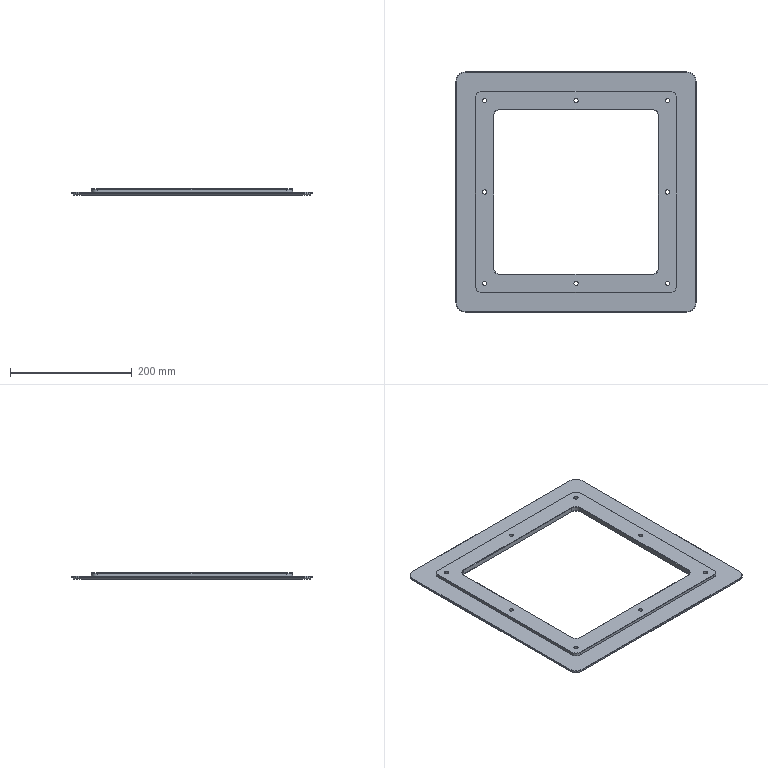NC program | Mastercam | posted with a generic post
Lines 1 to 950 of 5147:
%
O0000()
(MATERIAL - ALUMINUM MM - 2024)
( T14 | 20 FEM | H14 )
( T8 | 8 FEM | H8 | XY STOCK TO LEAVE - 0. | Z STOCK TO LEAVE - .1 )
( T12 | 12 FEM | H12 )
( T7 | 10 CHM | H7 )
( T24 | 63 FEM | H24 | XY STOCK TO LEAVE - -10. | Z STOCK TO LEAVE - 0. )
N100 G21
N110 G0 G17 G40 G49 G80 G90
N120 T14 M6
N130 G0 G90 G54 X-91.5 Y83. A0. S1600 M3
N140 G43 H14 Z50. M8
N150 Z2.
N160 G1 Z1. F600.
N170 X-89.5 F3000.
N180 G3 X-87.5 Y85. I0. J2.
N190 X-95. Y92.5 Z.925 I-7.5 J0.
N200 X-102.5 Y85. Z.85 I0. J-7.5
N210 X-95. Y77.5 Z.775 I7.5 J0.
N220 X-87.5 Y85. Z.7 I0. J7.5
N230 X-95. Y92.5 Z.625 I-7.5 J0.
N240 X-102.5 Y85. Z.55 I0. J-7.5
N250 X-95. Y77.5 Z.475 I7.5 J0.
N260 X-87.5 Y85. Z.4 I0. J7.5
N270 X-95. Y92.5 Z.325 I-7.5 J0.
N280 X-102.5 Y85. Z.25 I0. J-7.5
N290 X-95. Y77.5 Z.175 I7.5 J0.
N300 X-87.5 Y85. Z.1 I0. J7.5
N310 X-95. Y92.5 Z.025 I-7.5 J0.
N320 X-102.5 Y85. Z-.05 I0. J-7.5
N330 X-95. Y77.5 Z-.125 I7.5 J0.
N340 X-87.5 Y85. Z-.2 I0. J7.5
N350 X-95. Y92.5 Z-.275 I-7.5 J0.
N360 X-102.5 Y85. Z-.35 I0. J-7.5
N370 X-95. Y77.5 Z-.425 I7.5 J0.
N380 X-87.5 Y85. Z-.5 I0. J7.5
N390 X-95. Y92.5 Z-.575 I-7.5 J0.
N400 X-102.5 Y85. Z-.65 I0. J-7.5
N410 X-95. Y77.5 Z-.725 I7.5 J0.
N420 X-87.5 Y85. Z-.8 I0. J7.5
N430 X-95. Y92.5 Z-.875 I-7.5 J0.
N440 X-102.5 Y85. Z-.95 I0. J-7.5
N450 X-95. Y77.5 Z-1.025 I7.5 J0.
N460 X-87.5 Y85. Z-1.1 I0. J7.5
N470 X-95. Y92.5 Z-1.175 I-7.5 J0.
N480 X-102.5 Y85. Z-1.25 I0. J-7.5
N490 X-95. Y77.5 Z-1.325 I7.5 J0.
N500 X-87.5 Y85. Z-1.4 I0. J7.5
N510 X-95. Y92.5 Z-1.475 I-7.5 J0.
N520 X-102.5 Y85. Z-1.55 I0. J-7.5
N530 X-95. Y77.5 Z-1.625 I7.5 J0.
N540 X-87.5 Y85. Z-1.7 I0. J7.5
N550 X-95. Y92.5 Z-1.775 I-7.5 J0.
N560 X-102.5 Y85. Z-1.85 I0. J-7.5
N570 X-95. Y77.5 Z-1.925 I7.5 J0.
N580 X-87.5 Y85. Z-2. I0. J7.5
N590 X-95. Y92.5 I-7.5 J0.
N600 X-102.5 Y85. I0. J-7.5
N610 X-95. Y77.5 I7.5 J0.
N620 X-87.5 Y85. I0. J7.5
N630 X-89.5 Y87. I-2. J0.
N640 G1 X-91.5
N650 G0 Z50.
N660 Y-87.
N670 Z2.
N680 G1 Z1. F600.
N690 X-89.5 F3000.
N700 G3 X-87.5 Y-85. I0. J2.
N710 X-95. Y-77.5 Z.925 I-7.5 J0.
N720 X-102.5 Y-85. Z.85 I0. J-7.5
N730 X-95. Y-92.5 Z.775 I7.5 J0.
N740 X-87.5 Y-85. Z.7 I0. J7.5
N750 X-95. Y-77.5 Z.625 I-7.5 J0.
N760 X-102.5 Y-85. Z.55 I0. J-7.5
N770 X-95. Y-92.5 Z.475 I7.5 J0.
N780 X-87.5 Y-85. Z.4 I0. J7.5
N790 X-95. Y-77.5 Z.325 I-7.5 J0.
N800 X-102.5 Y-85. Z.25 I0. J-7.5
N810 X-95. Y-92.5 Z.175 I7.5 J0.
N820 X-87.5 Y-85. Z.1 I0. J7.5
N830 X-95. Y-77.5 Z.025 I-7.5 J0.
N840 X-102.5 Y-85. Z-.05 I0. J-7.5
N850 X-95. Y-92.5 Z-.125 I7.5 J0.
N860 X-87.5 Y-85. Z-.2 I0. J7.5
N870 X-95. Y-77.5 Z-.275 I-7.5 J0.
N880 X-102.5 Y-85. Z-.35 I0. J-7.5
N890 X-95. Y-92.5 Z-.425 I7.5 J0.
N900 X-87.5 Y-85. Z-.5 I0. J7.5
N910 X-95. Y-77.5 Z-.575 I-7.5 J0.
N920 X-102.5 Y-85. Z-.65 I0. J-7.5
N930 X-95. Y-92.5 Z-.725 I7.5 J0.
N940 X-87.5 Y-85. Z-.8 I0. J7.5
N950 X-95. Y-77.5 Z-.875 I-7.5 J0.
N960 X-102.5 Y-85. Z-.95 I0. J-7.5
N970 X-95. Y-92.5 Z-1.025 I7.5 J0.
N980 X-87.5 Y-85. Z-1.1 I0. J7.5
N990 X-95. Y-77.5 Z-1.175 I-7.5 J0.
N1000 X-102.5 Y-85. Z-1.25 I0. J-7.5
N1010 X-95. Y-92.5 Z-1.325 I7.5 J0.
N1020 X-87.5 Y-85. Z-1.4 I0. J7.5
N1030 X-95. Y-77.5 Z-1.475 I-7.5 J0.
N1040 X-102.5 Y-85. Z-1.55 I0. J-7.5
N1050 X-95. Y-92.5 Z-1.625 I7.5 J0.
N1060 X-87.5 Y-85. Z-1.7 I0. J7.5
N1070 X-95. Y-77.5 Z-1.775 I-7.5 J0.
N1080 X-102.5 Y-85. Z-1.85 I0. J-7.5
N1090 X-95. Y-92.5 Z-1.925 I7.5 J0.
N1100 X-87.5 Y-85. Z-2. I0. J7.5
N1110 X-95. Y-77.5 I-7.5 J0.
N1120 X-102.5 Y-85. I0. J-7.5
N1130 X-95. Y-92.5 I7.5 J0.
N1140 X-87.5 Y-85. I0. J7.5
N1150 X-89.5 Y-83. I-2. J0.
N1160 G1 X-91.5
N1170 G0 Z50.
N1180 X98.5 Y-87.
N1190 Z2.
N1200 G1 Z1. F600.
N1210 X100.5 F3000.
N1220 G3 X102.5 Y-85. I0. J2.
N1230 X95. Y-77.5 Z.925 I-7.5 J0.
N1240 X87.5 Y-85. Z.85 I0. J-7.5
N1250 X95. Y-92.5 Z.775 I7.5 J0.
N1260 X102.5 Y-85. Z.7 I0. J7.5
N1270 X95. Y-77.5 Z.625 I-7.5 J0.
N1280 X87.5 Y-85. Z.55 I0. J-7.5
N1290 X95. Y-92.5 Z.475 I7.5 J0.
N1300 X102.5 Y-85. Z.4 I0. J7.5
N1310 X95. Y-77.5 Z.325 I-7.5 J0.
N1320 X87.5 Y-85. Z.25 I0. J-7.5
N1330 X95. Y-92.5 Z.175 I7.5 J0.
N1340 X102.5 Y-85. Z.1 I0. J7.5
N1350 X95. Y-77.5 Z.025 I-7.5 J0.
N1360 X87.5 Y-85. Z-.05 I0. J-7.5
N1370 X95. Y-92.5 Z-.125 I7.5 J0.
N1380 X102.5 Y-85. Z-.2 I0. J7.5
N1390 X95. Y-77.5 Z-.275 I-7.5 J0.
N1400 X87.5 Y-85. Z-.35 I0. J-7.5
N1410 X95. Y-92.5 Z-.425 I7.5 J0.
N1420 X102.5 Y-85. Z-.5 I0. J7.5
N1430 X95. Y-77.5 Z-.575 I-7.5 J0.
N1440 X87.5 Y-85. Z-.65 I0. J-7.5
N1450 X95. Y-92.5 Z-.725 I7.5 J0.
N1460 X102.5 Y-85. Z-.8 I0. J7.5
N1470 X95. Y-77.5 Z-.875 I-7.5 J0.
N1480 X87.5 Y-85. Z-.95 I0. J-7.5
N1490 X95. Y-92.5 Z-1.025 I7.5 J0.
N1500 X102.5 Y-85. Z-1.1 I0. J7.5
N1510 X95. Y-77.5 Z-1.175 I-7.5 J0.
N1520 X87.5 Y-85. Z-1.25 I0. J-7.5
N1530 X95. Y-92.5 Z-1.325 I7.5 J0.
N1540 X102.5 Y-85. Z-1.4 I0. J7.5
N1550 X95. Y-77.5 Z-1.475 I-7.5 J0.
N1560 X87.5 Y-85. Z-1.55 I0. J-7.5
N1570 X95. Y-92.5 Z-1.625 I7.5 J0.
N1580 X102.5 Y-85. Z-1.7 I0. J7.5
N1590 X95. Y-77.5 Z-1.775 I-7.5 J0.
N1600 X87.5 Y-85. Z-1.85 I0. J-7.5
N1610 X95. Y-92.5 Z-1.925 I7.5 J0.
N1620 X102.5 Y-85. Z-2. I0. J7.5
N1630 X95. Y-77.5 I-7.5 J0.
N1640 X87.5 Y-85. I0. J-7.5
N1650 X95. Y-92.5 I7.5 J0.
N1660 X102.5 Y-85. I0. J7.5
N1670 X100.5 Y-83. I-2. J0.
N1680 G1 X98.5
N1690 G0 Z50.
N1700 Y83.
N1710 Z2.
N1720 G1 Z1. F600.
N1730 X100.5 F3000.
N1740 G3 X102.5 Y85. I0. J2.
N1750 X95. Y92.5 Z.925 I-7.5 J0.
N1760 X87.5 Y85. Z.85 I0. J-7.5
N1770 X95. Y77.5 Z.775 I7.5 J0.
N1780 X102.5 Y85. Z.7 I0. J7.5
N1790 X95. Y92.5 Z.625 I-7.5 J0.
N1800 X87.5 Y85. Z.55 I0. J-7.5
N1810 X95. Y77.5 Z.475 I7.5 J0.
N1820 X102.5 Y85. Z.4 I0. J7.5
N1830 X95. Y92.5 Z.325 I-7.5 J0.
N1840 X87.5 Y85. Z.25 I0. J-7.5
N1850 X95. Y77.5 Z.175 I7.5 J0.
N1860 X102.5 Y85. Z.1 I0. J7.5
N1870 X95. Y92.5 Z.025 I-7.5 J0.
N1880 X87.5 Y85. Z-.05 I0. J-7.5
N1890 X95. Y77.5 Z-.125 I7.5 J0.
N1900 X102.5 Y85. Z-.2 I0. J7.5
N1910 X95. Y92.5 Z-.275 I-7.5 J0.
N1920 X87.5 Y85. Z-.35 I0. J-7.5
N1930 X95. Y77.5 Z-.425 I7.5 J0.
N1940 X102.5 Y85. Z-.5 I0. J7.5
N1950 X95. Y92.5 Z-.575 I-7.5 J0.
N1960 X87.5 Y85. Z-.65 I0. J-7.5
N1970 X95. Y77.5 Z-.725 I7.5 J0.
N1980 X102.5 Y85. Z-.8 I0. J7.5
N1990 X95. Y92.5 Z-.875 I-7.5 J0.
N2000 X87.5 Y85. Z-.95 I0. J-7.5
N2010 X95. Y77.5 Z-1.025 I7.5 J0.
N2020 X102.5 Y85. Z-1.1 I0. J7.5
N2030 X95. Y92.5 Z-1.175 I-7.5 J0.
N2040 X87.5 Y85. Z-1.25 I0. J-7.5
N2050 X95. Y77.5 Z-1.325 I7.5 J0.
N2060 X102.5 Y85. Z-1.4 I0. J7.5
N2070 X95. Y92.5 Z-1.475 I-7.5 J0.
N2080 X87.5 Y85. Z-1.55 I0. J-7.5
N2090 X95. Y77.5 Z-1.625 I7.5 J0.
N2100 X102.5 Y85. Z-1.7 I0. J7.5
N2110 X95. Y92.5 Z-1.775 I-7.5 J0.
N2120 X87.5 Y85. Z-1.85 I0. J-7.5
N2130 X95. Y77.5 Z-1.925 I7.5 J0.
N2140 X102.5 Y85. Z-2. I0. J7.5
N2150 X95. Y92.5 I-7.5 J0.
N2160 X87.5 Y85. I0. J-7.5
N2170 X95. Y77.5 I7.5 J0.
N2180 X102.5 Y85. I0. J7.5
N2190 X100.5 Y87. I-2. J0.
N2200 G1 X98.5
N2210 G0 Z50.
N2220 M5
N2230 G91 G28 Z0. M9
N2240 A0.
N2250 M01
N2260 T8 M6
N2270 G0 G90 G17 G54 X-94.1 Y84.2 A0. S3500 M3
N2280 G43 H8 Z50. M8
N2290 Z2.
N2300 G1 Z1. F600.
N2310 X-93.3 F1000.
N2320 G3 X-92.5 Y85. I0. J.8
N2330 X-95. Y87.5 Z.925 I-2.5 J0.
N2340 X-97.5 Y85. Z.85 I0. J-2.5
N2350 X-95. Y82.5 Z.775 I2.5 J0.
N2360 X-92.5 Y85. Z.7 I0. J2.5
N2370 X-95. Y87.5 Z.625 I-2.5 J0.
N2380 X-97.5 Y85. Z.55 I0. J-2.5
N2390 X-95. Y82.5 Z.475 I2.5 J0.
N2400 X-92.5 Y85. Z.4 I0. J2.5
N2410 X-95. Y87.5 Z.325 I-2.5 J0.
N2420 X-97.5 Y85. Z.25 I0. J-2.5
N2430 X-95. Y82.5 Z.175 I2.5 J0.
N2440 X-92.5 Y85. Z.1 I0. J2.5
N2450 X-95. Y87.5 Z.025 I-2.5 J0.
N2460 X-97.5 Y85. Z-.05 I0. J-2.5
N2470 X-95. Y82.5 Z-.125 I2.5 J0.
N2480 X-92.5 Y85. Z-.2 I0. J2.5
N2490 X-95. Y87.5 Z-.275 I-2.5 J0.
N2500 X-97.5 Y85. Z-.35 I0. J-2.5
N2510 X-95. Y82.5 Z-.425 I2.5 J0.
N2520 X-92.5 Y85. Z-.5 I0. J2.5
N2530 X-95. Y87.5 Z-.575 I-2.5 J0.
N2540 X-97.5 Y85. Z-.65 I0. J-2.5
N2550 X-95. Y82.5 Z-.725 I2.5 J0.
N2560 X-92.5 Y85. Z-.8 I0. J2.5
N2570 X-95. Y87.5 Z-.875 I-2.5 J0.
N2580 X-97.5 Y85. Z-.95 I0. J-2.5
N2590 X-95. Y82.5 Z-1.025 I2.5 J0.
N2600 X-92.5 Y85. Z-1.1 I0. J2.5
N2610 X-95. Y87.5 Z-1.175 I-2.5 J0.
N2620 X-97.5 Y85. Z-1.25 I0. J-2.5
N2630 X-95. Y82.5 Z-1.325 I2.5 J0.
N2640 X-92.5 Y85. Z-1.4 I0. J2.5
N2650 X-95. Y87.5 Z-1.475 I-2.5 J0.
N2660 X-97.5 Y85. Z-1.55 I0. J-2.5
N2670 X-95. Y82.5 Z-1.625 I2.5 J0.
N2680 X-92.5 Y85. Z-1.7 I0. J2.5
N2690 X-95. Y87.5 Z-1.775 I-2.5 J0.
N2700 X-97.5 Y85. Z-1.85 I0. J-2.5
N2710 X-95. Y82.5 Z-1.925 I2.5 J0.
N2720 X-92.5 Y85. Z-2. I0. J2.5
N2730 X-95. Y87.5 Z-2.075 I-2.5 J0.
N2740 X-97.5 Y85. Z-2.15 I0. J-2.5
N2750 X-95. Y82.5 Z-2.225 I2.5 J0.
N2760 X-92.5 Y85. Z-2.3 I0. J2.5
N2770 X-95. Y87.5 Z-2.375 I-2.5 J0.
N2780 X-97.5 Y85. Z-2.45 I0. J-2.5
N2790 X-95. Y82.5 Z-2.525 I2.5 J0.
N2800 X-92.5 Y85. Z-2.6 I0. J2.5
N2810 X-95. Y87.5 Z-2.675 I-2.5 J0.
N2820 X-97.5 Y85. Z-2.75 I0. J-2.5
N2830 X-95. Y82.5 Z-2.825 I2.5 J0.
N2840 X-92.5 Y85. Z-2.9 I0. J2.5
N2850 X-95. Y87.5 Z-2.975 I-2.5 J0.
N2860 X-97.5 Y85. Z-3.05 I0. J-2.5
N2870 X-95. Y82.5 Z-3.125 I2.5 J0.
N2880 X-92.5 Y85. Z-3.2 I0. J2.5
N2890 X-95. Y87.5 Z-3.275 I-2.5 J0.
N2900 X-97.5 Y85. Z-3.35 I0. J-2.5
N2910 X-95. Y82.5 Z-3.425 I2.5 J0.
N2920 X-92.5 Y85. Z-3.5 I0. J2.5
N2930 X-95. Y87.5 Z-3.575 I-2.5 J0.
N2940 X-97.5 Y85. Z-3.65 I0. J-2.5
N2950 X-95. Y82.5 Z-3.725 I2.5 J0.
N2960 X-92.5 Y85. Z-3.8 I0. J2.5
N2970 X-95. Y87.5 Z-3.875 I-2.5 J0.
N2980 X-97.5 Y85. Z-3.95 I0. J-2.5
N2990 X-95. Y82.5 Z-4.025 I2.5 J0.
N3000 X-92.5 Y85. Z-4.1 I0. J2.5
N3010 X-95. Y87.5 Z-4.175 I-2.5 J0.
N3020 X-97.5 Y85. Z-4.25 I0. J-2.5
N3030 X-95. Y82.5 Z-4.325 I2.5 J0.
N3040 X-92.5 Y85. Z-4.4 I0. J2.5
N3050 X-95. Y87.5 Z-4.475 I-2.5 J0.
N3060 X-97.5 Y85. Z-4.55 I0. J-2.5
N3070 X-95. Y82.5 Z-4.625 I2.5 J0.
N3080 X-92.5 Y85. Z-4.7 I0. J2.5
N3090 X-95. Y87.5 Z-4.775 I-2.5 J0.
N3100 X-97.5 Y85. Z-4.85 I0. J-2.5
N3110 X-95. Y82.5 Z-4.925 I2.5 J0.
N3120 X-92.5 Y85. Z-5. I0. J2.5
N3130 X-95. Y87.5 Z-5.075 I-2.5 J0.
N3140 X-97.5 Y85. Z-5.15 I0. J-2.5
N3150 X-95. Y82.5 Z-5.225 I2.5 J0.
N3160 X-92.5 Y85. Z-5.3 I0. J2.5
N3170 X-95. Y87.5 Z-5.375 I-2.5 J0.
N3180 X-97.5 Y85. Z-5.45 I0. J-2.5
N3190 X-95. Y82.5 Z-5.525 I2.5 J0.
N3200 X-92.5 Y85. Z-5.6 I0. J2.5
N3210 X-95. Y87.5 Z-5.675 I-2.5 J0.
N3220 X-97.5 Y85. Z-5.75 I0. J-2.5
N3230 X-95. Y82.5 Z-5.825 I2.5 J0.
N3240 X-92.5 Y85. Z-5.9 I0. J2.5
N3250 X-95. Y87.5 Z-5.975 I-2.5 J0.
N3260 X-97.5 Y85. Z-6.05 I0. J-2.5
N3270 X-95. Y82.5 Z-6.125 I2.5 J0.
N3280 X-92.5 Y85. Z-6.2 I0. J2.5
N3290 X-95. Y87.5 Z-6.275 I-2.5 J0.
N3300 X-97.5 Y85. Z-6.35 I0. J-2.5
N3310 X-95. Y82.5 Z-6.425 I2.5 J0.
N3320 X-92.5 Y85. Z-6.5 I0. J2.5
N3330 X-95. Y87.5 Z-6.575 I-2.5 J0.
N3340 X-97.5 Y85. Z-6.65 I0. J-2.5
N3350 X-95. Y82.5 Z-6.725 I2.5 J0.
N3360 X-92.5 Y85. Z-6.8 I0. J2.5
N3370 X-95. Y87.5 Z-6.875 I-2.5 J0.
N3380 X-97.5 Y85. Z-6.95 I0. J-2.5
N3390 X-95. Y82.5 Z-7.025 I2.5 J0.
N3400 X-92.5 Y85. Z-7.1 I0. J2.5
N3410 X-95. Y87.5 Z-7.175 I-2.5 J0.
N3420 X-97.5 Y85. Z-7.25 I0. J-2.5
N3430 X-95. Y82.5 Z-7.325 I2.5 J0.
N3440 X-92.5 Y85. Z-7.4 I0. J2.5
N3450 X-95. Y87.5 Z-7.475 I-2.5 J0.
N3460 X-97.5 Y85. Z-7.55 I0. J-2.5
N3470 X-95. Y82.5 Z-7.625 I2.5 J0.
N3480 X-92.5 Y85. Z-7.7 I0. J2.5
N3490 X-95. Y87.5 Z-7.775 I-2.5 J0.
N3500 X-97.5 Y85. Z-7.85 I0. J-2.5
N3510 X-95. Y82.5 Z-7.925 I2.5 J0.
N3520 X-92.5 Y85. Z-8. I0. J2.5
N3530 X-95. Y87.5 Z-8.075 I-2.5 J0.
N3540 X-97.5 Y85. Z-8.15 I0. J-2.5
N3550 X-95. Y82.5 Z-8.225 I2.5 J0.
N3560 X-92.5 Y85. Z-8.3 I0. J2.5
N3570 X-95. Y87.5 Z-8.375 I-2.5 J0.
N3580 X-97.5 Y85. Z-8.45 I0. J-2.5
N3590 X-95. Y82.5 Z-8.525 I2.5 J0.
N3600 X-92.5 Y85. Z-8.6 I0. J2.5
N3610 X-95. Y87.5 Z-8.675 I-2.5 J0.
N3620 X-97.5 Y85. Z-8.75 I0. J-2.5
N3630 X-95. Y82.5 Z-8.825 I2.5 J0.
N3640 X-92.5 Y85. Z-8.9 I0. J2.5
N3650 X-95. Y87.5 Z-8.975 I-2.5 J0.
N3660 X-97.5 Y85. Z-9.05 I0. J-2.5
N3670 X-95. Y82.5 Z-9.125 I2.5 J0.
N3680 X-92.5 Y85. Z-9.2 I0. J2.5
N3690 X-95. Y87.5 Z-9.275 I-2.5 J0.
N3700 X-97.5 Y85. Z-9.35 I0. J-2.5
N3710 X-95. Y82.5 Z-9.425 I2.5 J0.
N3720 X-92.5 Y85. Z-9.5 I0. J2.5
N3730 X-95. Y87.5 Z-9.575 I-2.5 J0.
N3740 X-97.5 Y85. Z-9.65 I0. J-2.5
N3750 X-95. Y82.5 Z-9.725 I2.5 J0.
N3760 X-92.5 Y85. Z-9.8 I0. J2.5
N3770 X-95. Y87.5 Z-9.875 I-2.5 J0.
N3780 X-97.5 Y85. Z-9.95 I0. J-2.5
N3790 X-95. Y82.5 Z-10.025 I2.5 J0.
N3800 X-92.5 Y85. Z-10.1 I0. J2.5
N3810 X-95. Y87.5 Z-10.175 I-2.5 J0.
N3820 X-97.5 Y85. Z-10.25 I0. J-2.5
N3830 X-95. Y82.5 Z-10.325 I2.5 J0.
N3840 X-92.5 Y85. Z-10.4 I0. J2.5
N3850 X-95. Y87.5 Z-10.475 I-2.5 J0.
N3860 X-97.5 Y85. Z-10.55 I0. J-2.5
N3870 X-95. Y82.5 Z-10.625 I2.5 J0.
N3880 X-92.5 Y85. Z-10.7 I0. J2.5
N3890 X-95. Y87.5 Z-10.775 I-2.5 J0.
N3900 X-97.5 Y85. Z-10.85 I0. J-2.5
N3910 X-95. Y82.5 Z-10.925 I2.5 J0.
N3920 X-92.5 Y85. Z-11. I0. J2.5
N3930 X-95. Y87.5 Z-11.075 I-2.5 J0.
N3940 X-97.5 Y85. Z-11.15 I0. J-2.5
N3950 X-95. Y82.5 Z-11.225 I2.5 J0.
N3960 X-92.5 Y85. Z-11.3 I0. J2.5
N3970 X-95. Y87.5 Z-11.375 I-2.5 J0.
N3980 X-96.25 Y87.165 Z-11.4 I0. J-2.5
N3990 X-97.5 Y85. I1.25 J-2.165
N4000 X-95. Y82.5 I2.5 J0.
N4010 X-92.5 Y85. I0. J2.5
N4020 X-95. Y87.5 I-2.5 J0.
N4030 X-96.25 Y87.165 I0. J-2.5
N4040 X-96.65 Y86.472 I.4 J-.693
N4050 X-96.543 Y86.072 I.8 J0.
N4060 G1 X-96.143 Y85.379
N4070 G0 Z50.
N4080 X95.9 Y-85.8
N4090 Z2.
N4100 G1 Z1. F600.
N4110 X96.7 F1000.
N4120 G3 X97.5 Y-85. I0. J.8
N4130 X95. Y-82.5 Z.925 I-2.5 J0.
N4140 X92.5 Y-85. Z.85 I0. J-2.5
N4150 X95. Y-87.5 Z.775 I2.5 J0.
N4160 X97.5 Y-85. Z.7 I0. J2.5
N4170 X95. Y-82.5 Z.625 I-2.5 J0.
N4180 X92.5 Y-85. Z.55 I0. J-2.5
N4190 X95. Y-87.5 Z.475 I2.5 J0.
N4200 X97.5 Y-85. Z.4 I0. J2.5
N4210 X95. Y-82.5 Z.325 I-2.5 J0.
N4220 X92.5 Y-85. Z.25 I0. J-2.5
N4230 X95. Y-87.5 Z.175 I2.5 J0.
N4240 X97.5 Y-85. Z.1 I0. J2.5
N4250 X95. Y-82.5 Z.025 I-2.5 J0.
N4260 X92.5 Y-85. Z-.05 I0. J-2.5
N4270 X95. Y-87.5 Z-.125 I2.5 J0.
N4280 X97.5 Y-85. Z-.2 I0. J2.5
N4290 X95. Y-82.5 Z-.275 I-2.5 J0.
N4300 X92.5 Y-85. Z-.35 I0. J-2.5
N4310 X95. Y-87.5 Z-.425 I2.5 J0.
N4320 X97.5 Y-85. Z-.5 I0. J2.5
N4330 X95. Y-82.5 Z-.575 I-2.5 J0.
N4340 X92.5 Y-85. Z-.65 I0. J-2.5
N4350 X95. Y-87.5 Z-.725 I2.5 J0.
N4360 X97.5 Y-85. Z-.8 I0. J2.5
N4370 X95. Y-82.5 Z-.875 I-2.5 J0.
N4380 X92.5 Y-85. Z-.95 I0. J-2.5
N4390 X95. Y-87.5 Z-1.025 I2.5 J0.
N4400 X97.5 Y-85. Z-1.1 I0. J2.5
N4410 X95. Y-82.5 Z-1.175 I-2.5 J0.
N4420 X92.5 Y-85. Z-1.25 I0. J-2.5
N4430 X95. Y-87.5 Z-1.325 I2.5 J0.
N4440 X97.5 Y-85. Z-1.4 I0. J2.5
N4450 X95. Y-82.5 Z-1.475 I-2.5 J0.
N4460 X92.5 Y-85. Z-1.55 I0. J-2.5
N4470 X95. Y-87.5 Z-1.625 I2.5 J0.
N4480 X97.5 Y-85. Z-1.7 I0. J2.5
N4490 X95. Y-82.5 Z-1.775 I-2.5 J0.
N4500 X92.5 Y-85. Z-1.85 I0. J-2.5
N4510 X95. Y-87.5 Z-1.925 I2.5 J0.
N4520 X97.5 Y-85. Z-2. I0. J2.5
N4530 X95. Y-82.5 Z-2.075 I-2.5 J0.
N4540 X92.5 Y-85. Z-2.15 I0. J-2.5
N4550 X95. Y-87.5 Z-2.225 I2.5 J0.
N4560 X97.5 Y-85. Z-2.3 I0. J2.5
N4570 X95. Y-82.5 Z-2.375 I-2.5 J0.
N4580 X92.5 Y-85. Z-2.45 I0. J-2.5
N4590 X95. Y-87.5 Z-2.525 I2.5 J0.
N4600 X97.5 Y-85. Z-2.6 I0. J2.5
N4610 X95. Y-82.5 Z-2.675 I-2.5 J0.
N4620 X92.5 Y-85. Z-2.75 I0. J-2.5
N4630 X95. Y-87.5 Z-2.825 I2.5 J0.
N4640 X97.5 Y-85. Z-2.9 I0. J2.5
N4650 X95. Y-82.5 Z-2.975 I-2.5 J0.
N4660 X92.5 Y-85. Z-3.05 I0. J-2.5
N4670 X95. Y-87.5 Z-3.125 I2.5 J0.
N4680 X97.5 Y-85. Z-3.2 I0. J2.5
N4690 X95. Y-82.5 Z-3.275 I-2.5 J0.
N4700 X92.5 Y-85. Z-3.35 I0. J-2.5
N4710 X95. Y-87.5 Z-3.425 I2.5 J0.
N4720 X97.5 Y-85. Z-3.5 I0. J2.5
N4730 X95. Y-82.5 Z-3.575 I-2.5 J0.
N4740 X92.5 Y-85. Z-3.65 I0. J-2.5
N4750 X95. Y-87.5 Z-3.725 I2.5 J0.
N4760 X97.5 Y-85. Z-3.8 I0. J2.5
N4770 X95. Y-82.5 Z-3.875 I-2.5 J0.
N4780 X92.5 Y-85. Z-3.95 I0. J-2.5
N4790 X95. Y-87.5 Z-4.025 I2.5 J0.
N4800 X97.5 Y-85. Z-4.1 I0. J2.5
N4810 X95. Y-82.5 Z-4.175 I-2.5 J0.
N4820 X92.5 Y-85. Z-4.25 I0. J-2.5
N4830 X95. Y-87.5 Z-4.325 I2.5 J0.
N4840 X97.5 Y-85. Z-4.4 I0. J2.5
N4850 X95. Y-82.5 Z-4.475 I-2.5 J0.
N4860 X92.5 Y-85. Z-4.55 I0. J-2.5
N4870 X95. Y-87.5 Z-4.625 I2.5 J0.
N4880 X97.5 Y-85. Z-4.7 I0. J2.5
N4890 X95. Y-82.5 Z-4.775 I-2.5 J0.
N4900 X92.5 Y-85. Z-4.85 I0. J-2.5
N4910 X95. Y-87.5 Z-4.925 I2.5 J0.
N4920 X97.5 Y-85. Z-5. I0. J2.5
N4930 X95. Y-82.5 Z-5.075 I-2.5 J0.
N4940 X92.5 Y-85. Z-5.15 I0. J-2.5
N4950 X95. Y-87.5 Z-5.225 I2.5 J0.
N4960 X97.5 Y-85. Z-5.3 I0. J2.5
N4970 X95. Y-82.5 Z-5.375 I-2.5 J0.
N4980 X92.5 Y-85. Z-5.45 I0. J-2.5
N4990 X95. Y-87.5 Z-5.525 I2.5 J0.
N5000 X97.5 Y-85. Z-5.6 I0. J2.5
N5010 X95. Y-82.5 Z-5.675 I-2.5 J0.
N5020 X92.5 Y-85. Z-5.75 I0. J-2.5
N5030 X95. Y-87.5 Z-5.825 I2.5 J0.
N5040 X97.5 Y-85. Z-5.9 I0. J2.5
N5050 X95. Y-82.5 Z-5.975 I-2.5 J0.
N5060 X92.5 Y-85. Z-6.05 I0. J-2.5
N5070 X95. Y-87.5 Z-6.125 I2.5 J0.
N5080 X97.5 Y-85. Z-6.2 I0. J2.5
N5090 X95. Y-82.5 Z-6.275 I-2.5 J0.
N5100 X92.5 Y-85. Z-6.35 I0. J-2.5
N5110 X95. Y-87.5 Z-6.425 I2.5 J0.
N5120 X97.5 Y-85. Z-6.5 I0. J2.5
N5130 X95. Y-82.5 Z-6.575 I-2.5 J0.
N5140 X92.5 Y-85. Z-6.65 I0. J-2.5
N5150 X95. Y-87.5 Z-6.725 I2.5 J0.
N5160 X97.5 Y-85. Z-6.8 I0. J2.5
N5170 X95. Y-82.5 Z-6.875 I-2.5 J0.
N5180 X92.5 Y-85. Z-6.95 I0. J-2.5
N5190 X95. Y-87.5 Z-7.025 I2.5 J0.
N5200 X97.5 Y-85. Z-7.1 I0. J2.5
N5210 X95. Y-82.5 Z-7.175 I-2.5 J0.
N5220 X92.5 Y-85. Z-7.25 I0. J-2.5
N5230 X95. Y-87.5 Z-7.325 I2.5 J0.
N5240 X97.5 Y-85. Z-7.4 I0. J2.5
N5250 X95. Y-82.5 Z-7.475 I-2.5 J0.
N5260 X92.5 Y-85. Z-7.55 I0. J-2.5
N5270 X95. Y-87.5 Z-7.625 I2.5 J0.
N5280 X97.5 Y-85. Z-7.7 I0. J2.5
N5290 X95. Y-82.5 Z-7.775 I-2.5 J0.
N5300 X92.5 Y-85. Z-7.85 I0. J-2.5
N5310 X95. Y-87.5 Z-7.925 I2.5 J0.
N5320 X97.5 Y-85. Z-8. I0. J2.5
N5330 X95. Y-82.5 Z-8.075 I-2.5 J0.
N5340 X92.5 Y-85. Z-8.15 I0. J-2.5
N5350 X95. Y-87.5 Z-8.225 I2.5 J0.
N5360 X97.5 Y-85. Z-8.3 I0. J2.5
N5370 X95. Y-82.5 Z-8.375 I-2.5 J0.
N5380 X92.5 Y-85. Z-8.45 I0. J-2.5
N5390 X95. Y-87.5 Z-8.525 I2.5 J0.
N5400 X97.5 Y-85. Z-8.6 I0. J2.5
N5410 X95. Y-82.5 Z-8.675 I-2.5 J0.
N5420 X92.5 Y-85. Z-8.75 I0. J-2.5
N5430 X95. Y-87.5 Z-8.825 I2.5 J0.
N5440 X97.5 Y-85. Z-8.9 I0. J2.5
N5450 X95. Y-82.5 Z-8.975 I-2.5 J0.
N5460 X92.5 Y-85. Z-9.05 I0. J-2.5
N5470 X95. Y-87.5 Z-9.125 I2.5 J0.
N5480 X97.5 Y-85. Z-9.2 I0. J2.5
N5490 X95. Y-82.5 Z-9.275 I-2.5 J0.
N5500 X92.5 Y-85. Z-9.35 I0. J-2.5
N5510 X95. Y-87.5 Z-9.425 I2.5 J0.
N5520 X97.5 Y-85. Z-9.5 I0. J2.5
N5530 X95. Y-82.5 Z-9.575 I-2.5 J0.
N5540 X92.5 Y-85. Z-9.65 I0. J-2.5
N5550 X95. Y-87.5 Z-9.725 I2.5 J0.
N5560 X97.5 Y-85. Z-9.8 I0. J2.5
N5570 X95. Y-82.5 Z-9.875 I-2.5 J0.
N5580 X92.5 Y-85. Z-9.95 I0. J-2.5
N5590 X95. Y-87.5 Z-10.025 I2.5 J0.
N5600 X97.5 Y-85. Z-10.1 I0. J2.5
N5610 X95. Y-82.5 Z-10.175 I-2.5 J0.
N5620 X92.5 Y-85. Z-10.25 I0. J-2.5
N5630 X95. Y-87.5 Z-10.325 I2.5 J0.
N5640 X97.5 Y-85. Z-10.4 I0. J2.5
N5650 X95. Y-82.5 Z-10.475 I-2.5 J0.
N5660 X92.5 Y-85. Z-10.55 I0. J-2.5
N5670 X95. Y-87.5 Z-10.625 I2.5 J0.
N5680 X97.5 Y-85. Z-10.7 I0. J2.5
N5690 X95. Y-82.5 Z-10.775 I-2.5 J0.
N5700 X92.5 Y-85. Z-10.85 I0. J-2.5
N5710 X95. Y-87.5 Z-10.925 I2.5 J0.
N5720 X97.5 Y-85. Z-11. I0. J2.5
N5730 X95. Y-82.5 Z-11.075 I-2.5 J0.
N5740 X92.5 Y-85. Z-11.15 I0. J-2.5
N5750 X95. Y-87.5 Z-11.225 I2.5 J0.
N5760 X97.5 Y-85. Z-11.3 I0. J2.5
N5770 X95. Y-82.5 Z-11.375 I-2.5 J0.
N5780 X93.75 Y-82.835 Z-11.4 I0. J-2.5
N5790 X92.5 Y-85. I1.25 J-2.165
N5800 X95. Y-87.5 I2.5 J0.
N5810 X97.5 Y-85. I0. J2.5
N5820 X95. Y-82.5 I-2.5 J0.
N5830 X93.75 Y-82.835 I0. J-2.5
N5840 X93.35 Y-83.528 I.4 J-.693
N5850 X93.457 Y-83.928 I.8 J0.
N5860 G1 X93.857 Y-84.621
N5870 G0 Z50.
N5880 X-94.1 Y-85.8
N5890 Z2.
N5900 G1 Z1. F600.
N5910 X-93.3 F1000.
N5920 G3 X-92.5 Y-85. I0. J.8
N5930 X-95. Y-82.5 Z.925 I-2.5 J0.
N5940 X-97.5 Y-85. Z.85 I0. J-2.5
N5950 X-95. Y-87.5 Z.775 I2.5 J0.
N5960 X-92.5 Y-85. Z.7 I0. J2.5
N5970 X-95. Y-82.5 Z.625 I-2.5 J0.
N5980 X-97.5 Y-85. Z.55 I0. J-2.5
N5990 X-95. Y-87.5 Z.475 I2.5 J0.
N6000 X-92.5 Y-85. Z.4 I0. J2.5
N6010 X-95. Y-82.5 Z.325 I-2.5 J0.
N6020 X-97.5 Y-85. Z.25 I0. J-2.5
N6030 X-95. Y-87.5 Z.175 I2.5 J0.
N6040 X-92.5 Y-85. Z.1 I0. J2.5
N6050 X-95. Y-82.5 Z.025 I-2.5 J0.
N6060 X-97.5 Y-85. Z-.05 I0. J-2.5
N6070 X-95. Y-87.5 Z-.125 I2.5 J0.
N6080 X-92.5 Y-85. Z-.2 I0. J2.5
N6090 X-95. Y-82.5 Z-.275 I-2.5 J0.
N6100 X-97.5 Y-85. Z-.35 I0. J-2.5
N6110 X-95. Y-87.5 Z-.425 I2.5 J0.
N6120 X-92.5 Y-85. Z-.5 I0. J2.5
N6130 X-95. Y-82.5 Z-.575 I-2.5 J0.
N6140 X-97.5 Y-85. Z-.65 I0. J-2.5
N6150 X-95. Y-87.5 Z-.725 I2.5 J0.
N6160 X-92.5 Y-85. Z-.8 I0. J2.5
N6170 X-95. Y-82.5 Z-.875 I-2.5 J0.
N6180 X-97.5 Y-85. Z-.95 I0. J-2.5
N6190 X-95. Y-87.5 Z-1.025 I2.5 J0.
N6200 X-92.5 Y-85. Z-1.1 I0. J2.5
N6210 X-95. Y-82.5 Z-1.175 I-2.5 J0.
N6220 X-97.5 Y-85. Z-1.25 I0. J-2.5
N6230 X-95. Y-87.5 Z-1.325 I2.5 J0.
N6240 X-92.5 Y-85. Z-1.4 I0. J2.5
N6250 X-95. Y-82.5 Z-1.475 I-2.5 J0.
N6260 X-97.5 Y-85. Z-1.55 I0. J-2.5
N6270 X-95. Y-87.5 Z-1.625 I2.5 J0.
N6280 X-92.5 Y-85. Z-1.7 I0. J2.5
N6290 X-95. Y-82.5 Z-1.775 I-2.5 J0.
N6300 X-97.5 Y-85. Z-1.85 I0. J-2.5
N6310 X-95. Y-87.5 Z-1.925 I2.5 J0.
N6320 X-92.5 Y-85. Z-2. I0. J2.5
N6330 X-95. Y-82.5 Z-2.075 I-2.5 J0.
N6340 X-97.5 Y-85. Z-2.15 I0. J-2.5
N6350 X-95. Y-87.5 Z-2.225 I2.5 J0.
N6360 X-92.5 Y-85. Z-2.3 I0. J2.5
N6370 X-95. Y-82.5 Z-2.375 I-2.5 J0.
N6380 X-97.5 Y-85. Z-2.45 I0. J-2.5
N6390 X-95. Y-87.5 Z-2.525 I2.5 J0.
N6400 X-92.5 Y-85. Z-2.6 I0. J2.5
N6410 X-95. Y-82.5 Z-2.675 I-2.5 J0.
N6420 X-97.5 Y-85. Z-2.75 I0. J-2.5
N6430 X-95. Y-87.5 Z-2.825 I2.5 J0.
N6440 X-92.5 Y-85. Z-2.9 I0. J2.5
N6450 X-95. Y-82.5 Z-2.975 I-2.5 J0.
N6460 X-97.5 Y-85. Z-3.05 I0. J-2.5
N6470 X-95. Y-87.5 Z-3.125 I2.5 J0.
N6480 X-92.5 Y-85. Z-3.2 I0. J2.5
N6490 X-95. Y-82.5 Z-3.275 I-2.5 J0.
N6500 X-97.5 Y-85. Z-3.35 I0. J-2.5
N6510 X-95. Y-87.5 Z-3.425 I2.5 J0.
N6520 X-92.5 Y-85. Z-3.5 I0. J2.5
N6530 X-95. Y-82.5 Z-3.575 I-2.5 J0.
N6540 X-97.5 Y-85. Z-3.65 I0. J-2.5
N6550 X-95. Y-87.5 Z-3.725 I2.5 J0.
N6560 X-92.5 Y-85. Z-3.8 I0. J2.5
N6570 X-95. Y-82.5 Z-3.875 I-2.5 J0.
N6580 X-97.5 Y-85. Z-3.95 I0. J-2.5
N6590 X-95. Y-87.5 Z-4.025 I2.5 J0.
N6600 X-92.5 Y-85. Z-4.1 I0. J2.5
N6610 X-95. Y-82.5 Z-4.175 I-2.5 J0.
N6620 X-97.5 Y-85. Z-4.25 I0. J-2.5
N6630 X-95. Y-87.5 Z-4.325 I2.5 J0.
N6640 X-92.5 Y-85. Z-4.4 I0. J2.5
N6650 X-95. Y-82.5 Z-4.475 I-2.5 J0.
N6660 X-97.5 Y-85. Z-4.55 I0. J-2.5
N6670 X-95. Y-87.5 Z-4.625 I2.5 J0.
N6680 X-92.5 Y-85. Z-4.7 I0. J2.5
N6690 X-95. Y-82.5 Z-4.775 I-2.5 J0.
N6700 X-97.5 Y-85. Z-4.85 I0. J-2.5
N6710 X-95. Y-87.5 Z-4.925 I2.5 J0.
N6720 X-92.5 Y-85. Z-5. I0. J2.5
N6730 X-95. Y-82.5 Z-5.075 I-2.5 J0.
N6740 X-97.5 Y-85. Z-5.15 I0. J-2.5
N6750 X-95. Y-87.5 Z-5.225 I2.5 J0.
N6760 X-92.5 Y-85. Z-5.3 I0. J2.5
N6770 X-95. Y-82.5 Z-5.375 I-2.5 J0.
N6780 X-97.5 Y-85. Z-5.45 I0. J-2.5
N6790 X-95. Y-87.5 Z-5.525 I2.5 J0.
N6800 X-92.5 Y-85. Z-5.6 I0. J2.5
N6810 X-95. Y-82.5 Z-5.675 I-2.5 J0.
N6820 X-97.5 Y-85. Z-5.75 I0. J-2.5
N6830 X-95. Y-87.5 Z-5.825 I2.5 J0.
N6840 X-92.5 Y-85. Z-5.9 I0. J2.5
N6850 X-95. Y-82.5 Z-5.975 I-2.5 J0.
N6860 X-97.5 Y-85. Z-6.05 I0. J-2.5
N6870 X-95. Y-87.5 Z-6.125 I2.5 J0.
N6880 X-92.5 Y-85. Z-6.2 I0. J2.5
N6890 X-95. Y-82.5 Z-6.275 I-2.5 J0.
N6900 X-97.5 Y-85. Z-6.35 I0. J-2.5
N6910 X-95. Y-87.5 Z-6.425 I2.5 J0.
N6920 X-92.5 Y-85. Z-6.5 I0. J2.5
N6930 X-95. Y-82.5 Z-6.575 I-2.5 J0.
N6940 X-97.5 Y-85. Z-6.65 I0. J-2.5
N6950 X-95. Y-87.5 Z-6.725 I2.5 J0.
N6960 X-92.5 Y-85. Z-6.8 I0. J2.5
N6970 X-95. Y-82.5 Z-6.875 I-2.5 J0.
N6980 X-97.5 Y-85. Z-6.95 I0. J-2.5
N6990 X-95. Y-87.5 Z-7.025 I2.5 J0.
N7000 X-92.5 Y-85. Z-7.1 I0. J2.5
N7010 X-95. Y-82.5 Z-7.175 I-2.5 J0.
N7020 X-97.5 Y-85. Z-7.25 I0. J-2.5
N7030 X-95. Y-87.5 Z-7.325 I2.5 J0.
N7040 X-92.5 Y-85. Z-7.4 I0. J2.5
N7050 X-95. Y-82.5 Z-7.475 I-2.5 J0.
N7060 X-97.5 Y-85. Z-7.55 I0. J-2.5
N7070 X-95. Y-87.5 Z-7.625 I2.5 J0.
N7080 X-92.5 Y-85. Z-7.7 I0. J2.5
N7090 X-95. Y-82.5 Z-7.775 I-2.5 J0.
N7100 X-97.5 Y-85. Z-7.85 I0. J-2.5
N7110 X-95. Y-87.5 Z-7.925 I2.5 J0.
N7120 X-92.5 Y-85. Z-8. I0. J2.5
N7130 X-95. Y-82.5 Z-8.075 I-2.5 J0.
N7140 X-97.5 Y-85. Z-8.15 I0. J-2.5
N7150 X-95. Y-87.5 Z-8.225 I2.5 J0.
N7160 X-92.5 Y-85. Z-8.3 I0. J2.5
N7170 X-95. Y-82.5 Z-8.375 I-2.5 J0.
N7180 X-97.5 Y-85. Z-8.45 I0. J-2.5
N7190 X-95. Y-87.5 Z-8.525 I2.5 J0.
N7200 X-92.5 Y-85. Z-8.6 I0. J2.5
N7210 X-95. Y-82.5 Z-8.675 I-2.5 J0.
N7220 X-97.5 Y-85. Z-8.75 I0. J-2.5
N7230 X-95. Y-87.5 Z-8.825 I2.5 J0.
N7240 X-92.5 Y-85. Z-8.9 I0. J2.5
N7250 X-95. Y-82.5 Z-8.975 I-2.5 J0.
N7260 X-97.5 Y-85. Z-9.05 I0. J-2.5
N7270 X-95. Y-87.5 Z-9.125 I2.5 J0.
N7280 X-92.5 Y-85. Z-9.2 I0. J2.5
N7290 X-95. Y-82.5 Z-9.275 I-2.5 J0.
N7300 X-97.5 Y-85. Z-9.35 I0. J-2.5
N7310 X-95. Y-87.5 Z-9.425 I2.5 J0.
N7320 X-92.5 Y-85. Z-9.5 I0. J2.5
N7330 X-95. Y-82.5 Z-9.575 I-2.5 J0.
N7340 X-97.5 Y-85. Z-9.65 I0. J-2.5
N7350 X-95. Y-87.5 Z-9.725 I2.5 J0.
N7360 X-92.5 Y-85. Z-9.8 I0. J2.5
N7370 X-95. Y-82.5 Z-9.875 I-2.5 J0.
N7380 X-97.5 Y-85. Z-9.95 I0. J-2.5
N7390 X-95. Y-87.5 Z-10.025 I2.5 J0.
N7400 X-92.5 Y-85. Z-10.1 I0. J2.5
N7410 X-95. Y-82.5 Z-10.175 I-2.5 J0.
N7420 X-97.5 Y-85. Z-10.25 I0. J-2.5
N7430 X-95. Y-87.5 Z-10.325 I2.5 J0.
N7440 X-92.5 Y-85. Z-10.4 I0. J2.5
N7450 X-95. Y-82.5 Z-10.475 I-2.5 J0.
N7460 X-97.5 Y-85. Z-10.55 I0. J-2.5
N7470 X-95. Y-87.5 Z-10.625 I2.5 J0.
N7480 X-92.5 Y-85. Z-10.7 I0. J2.5
N7490 X-95. Y-82.5 Z-10.775 I-2.5 J0.
N7500 X-97.5 Y-85. Z-10.85 I0. J-2.5
N7510 X-95. Y-87.5 Z-10.925 I2.5 J0.
N7520 X-92.5 Y-85. Z-11. I0. J2.5
N7530 X-95. Y-82.5 Z-11.075 I-2.5 J0.
N7540 X-97.5 Y-85. Z-11.15 I0. J-2.5
N7550 X-95. Y-87.5 Z-11.225 I2.5 J0.
N7560 X-92.5 Y-85. Z-11.3 I0. J2.5
N7570 X-95. Y-82.5 Z-11.375 I-2.5 J0.
N7580 X-96.25 Y-82.835 Z-11.4 I0. J-2.5
N7590 X-97.5 Y-85. I1.25 J-2.165
N7600 X-95. Y-87.5 I2.5 J0.
N7610 X-92.5 Y-85. I0. J2.5
N7620 X-95. Y-82.5 I-2.5 J0.
N7630 X-96.25 Y-82.835 I0. J-2.5
N7640 X-96.65 Y-83.528 I.4 J-.693
N7650 X-96.543 Y-83.928 I.8 J0.
N7660 G1 X-96.143 Y-84.621
N7670 G0 Z50.
N7680 X95.9 Y84.2
N7690 Z2.
N7700 G1 Z1. F600.
N7710 X96.7 F1000.
N7720 G3 X97.5 Y85. I0. J.8
N7730 X95. Y87.5 Z.925 I-2.5 J0.
N7740 X92.5 Y85. Z.85 I0. J-2.5
N7750 X95. Y82.5 Z.775 I2.5 J0.
N7760 X97.5 Y85. Z.7 I0. J2.5
N7770 X95. Y87.5 Z.625 I-2.5 J0.
N7780 X92.5 Y85. Z.55 I0. J-2.5
N7790 X95. Y82.5 Z.475 I2.5 J0.
N7800 X97.5 Y85. Z.4 I0. J2.5
N7810 X95. Y87.5 Z.325 I-2.5 J0.
N7820 X92.5 Y85. Z.25 I0. J-2.5
N7830 X95. Y82.5 Z.175 I2.5 J0.
N7840 X97.5 Y85. Z.1 I0. J2.5
N7850 X95. Y87.5 Z.025 I-2.5 J0.
N7860 X92.5 Y85. Z-.05 I0. J-2.5
N7870 X95. Y82.5 Z-.125 I2.5 J0.
N7880 X97.5 Y85. Z-.2 I0. J2.5
N7890 X95. Y87.5 Z-.275 I-2.5 J0.
N7900 X92.5 Y85. Z-.35 I0. J-2.5
N7910 X95. Y82.5 Z-.425 I2.5 J0.
N7920 X97.5 Y85. Z-.5 I0. J2.5
N7930 X95. Y87.5 Z-.575 I-2.5 J0.
N7940 X92.5 Y85. Z-.65 I0. J-2.5
N7950 X95. Y82.5 Z-.725 I2.5 J0.
N7960 X97.5 Y85. Z-.8 I0. J2.5
N7970 X95. Y87.5 Z-.875 I-2.5 J0.
N7980 X92.5 Y85. Z-.95 I0. J-2.5
N7990 X95. Y82.5 Z-1.025 I2.5 J0.
N8000 X97.5 Y85. Z-1.1 I0. J2.5
N8010 X95. Y87.5 Z-1.175 I-2.5 J0.
N8020 X92.5 Y85. Z-1.25 I0. J-2.5
N8030 X95. Y82.5 Z-1.325 I2.5 J0.
N8040 X97.5 Y85. Z-1.4 I0. J2.5
N8050 X95. Y87.5 Z-1.475 I-2.5 J0.
N8060 X92.5 Y85. Z-1.55 I0. J-2.5
N8070 X95. Y82.5 Z-1.625 I2.5 J0.
N8080 X97.5 Y85. Z-1.7 I0. J2.5
N8090 X95. Y87.5 Z-1.775 I-2.5 J0.
N8100 X92.5 Y85. Z-1.85 I0. J-2.5
N8110 X95. Y82.5 Z-1.925 I2.5 J0.
N8120 X97.5 Y85. Z-2. I0. J2.5
N8130 X95. Y87.5 Z-2.075 I-2.5 J0.
N8140 X92.5 Y85. Z-2.15 I0. J-2.5
N8150 X95. Y82.5 Z-2.225 I2.5 J0.
N8160 X97.5 Y85. Z-2.3 I0. J2.5
N8170 X95. Y87.5 Z-2.375 I-2.5 J0.
N8180 X92.5 Y85. Z-2.45 I0. J-2.5
N8190 X95. Y82.5 Z-2.525 I2.5 J0.
N8200 X97.5 Y85. Z-2.6 I0. J2.5
N8210 X95. Y87.5 Z-2.675 I-2.5 J0.
N8220 X92.5 Y85. Z-2.75 I0. J-2.5
N8230 X95. Y82.5 Z-2.825 I2.5 J0.
N8240 X97.5 Y85. Z-2.9 I0. J2.5
N8250 X95. Y87.5 Z-2.975 I-2.5 J0.
N8260 X92.5 Y85. Z-3.05 I0. J-2.5
N8270 X95. Y82.5 Z-3.125 I2.5 J0.
N8280 X97.5 Y85. Z-3.2 I0. J2.5
N8290 X95. Y87.5 Z-3.275 I-2.5 J0.
N8300 X92.5 Y85. Z-3.35 I0. J-2.5
N8310 X95. Y82.5 Z-3.425 I2.5 J0.
N8320 X97.5 Y85. Z-3.5 I0. J2.5
N8330 X95. Y87.5 Z-3.575 I-2.5 J0.
N8340 X92.5 Y85. Z-3.65 I0. J-2.5
N8350 X95. Y82.5 Z-3.725 I2.5 J0.
N8360 X97.5 Y85. Z-3.8 I0. J2.5
N8370 X95. Y87.5 Z-3.875 I-2.5 J0.
N8380 X92.5 Y85. Z-3.95 I0. J-2.5
N8390 X95. Y82.5 Z-4.025 I2.5 J0.
N8400 X97.5 Y85. Z-4.1 I0. J2.5
N8410 X95. Y87.5 Z-4.175 I-2.5 J0.
N8420 X92.5 Y85. Z-4.25 I0. J-2.5
N8430 X95. Y82.5 Z-4.325 I2.5 J0.
N8440 X97.5 Y85. Z-4.4 I0. J2.5
N8450 X95. Y87.5 Z-4.475 I-2.5 J0.
N8460 X92.5 Y85. Z-4.55 I0. J-2.5
N8470 X95. Y82.5 Z-4.625 I2.5 J0.
N8480 X97.5 Y85. Z-4.7 I0. J2.5
N8490 X95. Y87.5 Z-4.775 I-2.5 J0.
N8500 X92.5 Y85. Z-4.85 I0. J-2.5
N8510 X95. Y82.5 Z-4.925 I2.5 J0.
N8520 X97.5 Y85. Z-5. I0. J2.5
N8530 X95. Y87.5 Z-5.075 I-2.5 J0.
N8540 X92.5 Y85. Z-5.15 I0. J-2.5
N8550 X95. Y82.5 Z-5.225 I2.5 J0.
N8560 X97.5 Y85. Z-5.3 I0. J2.5
N8570 X95. Y87.5 Z-5.375 I-2.5 J0.
N8580 X92.5 Y85. Z-5.45 I0. J-2.5
N8590 X95. Y82.5 Z-5.525 I2.5 J0.
N8600 X97.5 Y85. Z-5.6 I0. J2.5
N8610 X95. Y87.5 Z-5.675 I-2.5 J0.
N8620 X92.5 Y85. Z-5.75 I0. J-2.5
N8630 X95. Y82.5 Z-5.825 I2.5 J0.
N8640 X97.5 Y85. Z-5.9 I0. J2.5
N8650 X95. Y87.5 Z-5.975 I-2.5 J0.
N8660 X92.5 Y85. Z-6.05 I0. J-2.5
N8670 X95. Y82.5 Z-6.125 I2.5 J0.
N8680 X97.5 Y85. Z-6.2 I0. J2.5
N8690 X95. Y87.5 Z-6.275 I-2.5 J0.
N8700 X92.5 Y85. Z-6.35 I0. J-2.5
N8710 X95. Y82.5 Z-6.425 I2.5 J0.
N8720 X97.5 Y85. Z-6.5 I0. J2.5
N8730 X95. Y87.5 Z-6.575 I-2.5 J0.
N8740 X92.5 Y85. Z-6.65 I0. J-2.5
N8750 X95. Y82.5 Z-6.725 I2.5 J0.
N8760 X97.5 Y85. Z-6.8 I0. J2.5
N8770 X95. Y87.5 Z-6.875 I-2.5 J0.
N8780 X92.5 Y85. Z-6.95 I0. J-2.5
N8790 X95. Y82.5 Z-7.025 I2.5 J0.
N8800 X97.5 Y85. Z-7.1 I0. J2.5
N8810 X95. Y87.5 Z-7.175 I-2.5 J0.
N8820 X92.5 Y85. Z-7.25 I0. J-2.5
N8830 X95. Y82.5 Z-7.325 I2.5 J0.
N8840 X97.5 Y85. Z-7.4 I0. J2.5
N8850 X95. Y87.5 Z-7.475 I-2.5 J0.
N8860 X92.5 Y85. Z-7.55 I0. J-2.5
N8870 X95. Y82.5 Z-7.625 I2.5 J0.
N8880 X97.5 Y85. Z-7.7 I0. J2.5
N8890 X95. Y87.5 Z-7.775 I-2.5 J0.
N8900 X92.5 Y85. Z-7.85 I0. J-2.5
N8910 X95. Y82.5 Z-7.925 I2.5 J0.
N8920 X97.5 Y85. Z-8. I0. J2.5
N8930 X95. Y87.5 Z-8.075 I-2.5 J0.
N8940 X92.5 Y85. Z-8.15 I0. J-2.5
N8950 X95. Y82.5 Z-8.225 I2.5 J0.
N8960 X97.5 Y85. Z-8.3 I0. J2.5
N8970 X95. Y87.5 Z-8.375 I-2.5 J0.
N8980 X92.5 Y85. Z-8.45 I0. J-2.5
N8990 X95. Y82.5 Z-8.525 I2.5 J0.
N9000 X97.5 Y85. Z-8.6 I0. J2.5
N9010 X95. Y87.5 Z-8.675 I-2.5 J0.
N9020 X92.5 Y85. Z-8.75 I0. J-2.5
N9030 X95. Y82.5 Z-8.825 I2.5 J0.
N9040 X97.5 Y85. Z-8.9 I0. J2.5
N9050 X95. Y87.5 Z-8.975 I-2.5 J0.
N9060 X92.5 Y85. Z-9.05 I0. J-2.5
N9070 X95. Y82.5 Z-9.125 I2.5 J0.
N9080 X97.5 Y85. Z-9.2 I0. J2.5
N9090 X95. Y87.5 Z-9.275 I-2.5 J0.
N9100 X92.5 Y85. Z-9.35 I0. J-2.5
N9110 X95. Y82.5 Z-9.425 I2.5 J0.
N9120 X97.5 Y85. Z-9.5 I0. J2.5
N9130 X95. Y87.5 Z-9.575 I-2.5 J0.
N9140 X92.5 Y85. Z-9.65 I0. J-2.5
N9150 X95. Y82.5 Z-9.725 I2.5 J0.
N9160 X97.5 Y85. Z-9.8 I0. J2.5
N9170 X95. Y87.5 Z-9.875 I-2.5 J0.
N9180 X92.5 Y85. Z-9.95 I0. J-2.5
N9190 X95. Y82.5 Z-10.025 I2.5 J0.
N9200 X97.5 Y85. Z-10.1 I0. J2.5
N9210 X95. Y87.5 Z-10.175 I-2.5 J0.
N9220 X92.5 Y85. Z-10.25 I0. J-2.5
N9230 X95. Y82.5 Z-10.325 I2.5 J0.
N9240 X97.5 Y85. Z-10.4 I0. J2.5
N9250 X95. Y87.5 Z-10.475 I-2.5 J0.
N9260 X92.5 Y85. Z-10.55 I0. J-2.5
N9270 X95. Y82.5 Z-10.625 I2.5 J0.
N9280 X97.5 Y85. Z-10.7 I0. J2.5
N9290 X95. Y87.5 Z-10.775 I-2.5 J0.
N9300 X92.5 Y85. Z-10.85 I0. J-2.5
N9310 X95. Y82.5 Z-10.925 I2.5 J0.
N9320 X97.5 Y85. Z-11. I0. J2.5
N9330 X95. Y87.5 Z-11.075 I-2.5 J0.
N9340 X92.5 Y85. Z-11.15 I0. J-2.5
N9350 X95. Y82.5 Z-11.225 I2.5 J0.
N9360 X97.5 Y85. Z-11.3 I0. J2.5
N9370 X95. Y87.5 Z-11.375 I-2.5 J0.
N9380 X93.75 Y87.165 Z-11.4 I0. J-2.5
N9390 X92.5 Y85. I1.25 J-2.165
N9400 X95. Y82.5 I2.5 J0.
N9410 X97.5 Y85. I0. J2.5
N9420 X95. Y87.5 I-2.5 J0.
N9430 X93.75 Y87.165 I0. J-2.5
N9440 X93.35 Y86.472 I.4 J-.693
N9450 X93.457 Y86.072 I.8 J0.
N9460 G1 X93.857 Y85.379
N9470 G0 Z50.
N9480 M5
N9490 G91 G28 Z0. M9
N9500 A0.
N9510 M01